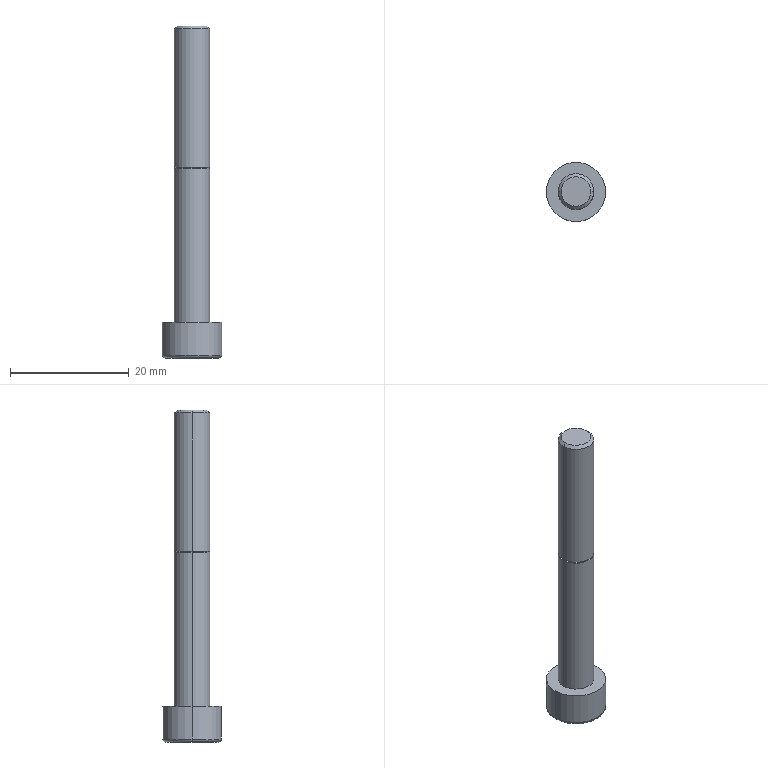Part | SolidWorks | features Attribute 1, Cut 1, Revolution 1 | 1 solid | 27 faces | box 10 x 10 x 56 mm | volume 1826 mm3 | plane 11 | torus 6 | cylinder 6 | cone 4 | commonest cylinder face diameters 6 x4 10 x2
STEP:
#1=CARTESIAN_POINT('',(-2.613,0.,26.01));
#2=VERTEX_POINT('',#1);
#3=CARTESIAN_POINT('',(-2.593,0.,26.03));
#4=VERTEX_POINT('',#3);
#5=CARTESIAN_POINT('',(-2.613,0.,26.03));
#6=DIRECTION('',(0.,-1.,0.));
#7=DIRECTION('',(0.,0.,-1.));
#8=AXIS2_PLACEMENT_3D('',#5,#6,#7);
#9=CIRCLE('',#8,0.02);
#10=EDGE_CURVE('',#2,#4,#9,.T.);
#11=ORIENTED_EDGE('',*,*,#10,.T.);
#12=CARTESIAN_POINT('',(2.593,0.,26.03));
#13=VERTEX_POINT('',#12);
#14=CARTESIAN_POINT('',(0.,0.,26.03));
#15=DIRECTION('',(0.,0.,-1.));
#16=DIRECTION('',(-1.,0.,0.));
#17=AXIS2_PLACEMENT_3D('',#14,#15,#16);
#18=CIRCLE('',#17,2.593);
#19=EDGE_CURVE('',#4,#13,#18,.T.);
#20=ORIENTED_EDGE('',*,*,#19,.T.);
#21=CARTESIAN_POINT('',(2.613,0.,26.01));
#22=VERTEX_POINT('',#21);
#23=CARTESIAN_POINT('',(2.613,0.,26.03));
#24=DIRECTION('',(0.,1.,0.));
#25=DIRECTION('',(-1.,0.,0.));
#26=AXIS2_PLACEMENT_3D('',#23,#24,#25);
#27=CIRCLE('',#26,0.02);
#28=EDGE_CURVE('',#22,#13,#27,.T.);
#29=ORIENTED_EDGE('',*,*,#28,.F.);
#30=CARTESIAN_POINT('',(0.,0.,26.01));
#31=DIRECTION('',(0.,0.,-1.));
#32=DIRECTION('',(-1.,0.,0.));
#33=AXIS2_PLACEMENT_3D('',#30,#31,#32);
#34=CIRCLE('',#33,2.613);
#35=EDGE_CURVE('',#2,#22,#34,.T.);
#36=ORIENTED_EDGE('',*,*,#35,.F.);
#37=EDGE_LOOP('',(#11,#20,#29,#36));
#38=FACE_OUTER_BOUND('',#37,.T.);
#39=CARTESIAN_POINT('',(0.,0.,26.03));
#40=DIRECTION('',(0.,0.,-1.));
#41=DIRECTION('',(-1.,0.,0.));
#42=AXIS2_PLACEMENT_3D('',#39,#40,#41);
#43=TOROIDAL_SURFACE('',#42,2.613,0.02);
#44=ADVANCED_FACE('',(#38),#43,.F.);
#45=ORIENTED_EDGE('',*,*,#28,.T.);
#46=CARTESIAN_POINT('',(0.,0.,26.03));
#47=DIRECTION('',(0.,0.,-1.));
#48=DIRECTION('',(-1.,0.,0.));
#49=AXIS2_PLACEMENT_3D('',#46,#47,#48);
#50=CIRCLE('',#49,2.593);
#51=EDGE_CURVE('',#13,#4,#50,.T.);
#52=ORIENTED_EDGE('',*,*,#51,.T.);
#53=ORIENTED_EDGE('',*,*,#10,.F.);
#54=CARTESIAN_POINT('',(0.,0.,26.01));
#55=DIRECTION('',(0.,0.,-1.));
#56=DIRECTION('',(-1.,0.,0.));
#57=AXIS2_PLACEMENT_3D('',#54,#55,#56);
#58=CIRCLE('',#57,2.613);
#59=EDGE_CURVE('',#22,#2,#58,.T.);
#60=ORIENTED_EDGE('',*,*,#59,.F.);
#61=EDGE_LOOP('',(#45,#52,#53,#60));
#62=FACE_OUTER_BOUND('',#61,.T.);
#63=CARTESIAN_POINT('',(0.,0.,26.03));
#64=DIRECTION('',(0.,0.,-1.));
#65=DIRECTION('',(-1.,0.,0.));
#66=AXIS2_PLACEMENT_3D('',#63,#64,#65);
#67=TOROIDAL_SURFACE('',#66,2.613,0.02);
#68=ADVANCED_FACE('',(#62),#67,.F.);
#69=CARTESIAN_POINT('',(-2.5,0.,50.));
#70=VERTEX_POINT('',#69);
#71=CARTESIAN_POINT('',(2.5,0.,50.));
#72=VERTEX_POINT('',#71);
#73=CARTESIAN_POINT('',(0.,0.,50.));
#74=DIRECTION('',(0.,0.,-1.));
#75=DIRECTION('',(-1.,0.,0.));
#76=AXIS2_PLACEMENT_3D('',#73,#74,#75);
#77=CIRCLE('',#76,2.5);
#78=EDGE_CURVE('',#70,#72,#77,.T.);
#79=ORIENTED_EDGE('',*,*,#78,.T.);
#80=CARTESIAN_POINT('',(3.,0.,49.5));
#81=VERTEX_POINT('',#80);
#82=CARTESIAN_POINT('',(2.5,0.,50.));
#83=DIRECTION('',(0.7071,0.,-0.7071));
#84=VECTOR('',#83,1000.);
#85=LINE('',#82,#84);
#86=EDGE_CURVE('',#72,#81,#85,.T.);
#87=ORIENTED_EDGE('',*,*,#86,.T.);
#88=CARTESIAN_POINT('',(-3.,0.,49.5));
#89=VERTEX_POINT('',#88);
#90=CARTESIAN_POINT('',(0.,0.,49.5));
#91=DIRECTION('',(0.,0.,-1.));
#92=DIRECTION('',(-1.,0.,0.));
#93=AXIS2_PLACEMENT_3D('',#90,#91,#92);
#94=CIRCLE('',#93,3.);
#95=EDGE_CURVE('',#89,#81,#94,.T.);
#96=ORIENTED_EDGE('',*,*,#95,.F.);
#97=CARTESIAN_POINT('',(-2.5,0.,50.));
#98=DIRECTION('',(-0.7071,0.,-0.7071));
#99=VECTOR('',#98,1000.);
#100=LINE('',#97,#99);
#101=EDGE_CURVE('',#70,#89,#100,.T.);
#102=ORIENTED_EDGE('',*,*,#101,.F.);
#103=EDGE_LOOP('',(#79,#87,#96,#102));
#104=FACE_OUTER_BOUND('',#103,.T.);
#105=CARTESIAN_POINT('',(0.,0.,50.));
#106=DIRECTION('',(0.,0.,-1.));
#107=DIRECTION('',(-1.,0.,0.));
#108=AXIS2_PLACEMENT_3D('',#105,#106,#107);
#109=CONICAL_SURFACE('',#108,2.5,0.7854);
#110=ADVANCED_FACE('',(#104),#109,.T.);
#111=ORIENTED_EDGE('',*,*,#95,.T.);
#112=CARTESIAN_POINT('',(3.,0.,26.192));
#113=VERTEX_POINT('',#112);
#114=CARTESIAN_POINT('',(3.,0.,-10.585));
#115=DIRECTION('',(0.,0.,-1.));
#116=VECTOR('',#115,1000.);
#117=LINE('',#114,#116);
#118=EDGE_CURVE('',#81,#113,#117,.T.);
#119=ORIENTED_EDGE('',*,*,#118,.T.);
#120=CARTESIAN_POINT('',(-3.,0.,26.192));
#121=VERTEX_POINT('',#120);
#122=CARTESIAN_POINT('',(0.,0.,26.192));
#123=DIRECTION('',(0.,0.,-1.));
#124=DIRECTION('',(-1.,0.,0.));
#125=AXIS2_PLACEMENT_3D('',#122,#123,#124);
#126=CIRCLE('',#125,3.);
#127=EDGE_CURVE('',#121,#113,#126,.T.);
#128=ORIENTED_EDGE('',*,*,#127,.F.);
#129=CARTESIAN_POINT('',(-3.,0.,-10.585));
#130=DIRECTION('',(0.,0.,-1.));
#131=VECTOR('',#130,1000.);
#132=LINE('',#129,#131);
#133=EDGE_CURVE('',#89,#121,#132,.T.);
#134=ORIENTED_EDGE('',*,*,#133,.F.);
#135=EDGE_LOOP('',(#111,#119,#128,#134));
#136=FACE_OUTER_BOUND('',#135,.T.);
#137=CARTESIAN_POINT('',(0.,0.,-10.585));
#138=DIRECTION('',(0.,0.,-1.));
#139=DIRECTION('',(-1.,0.,0.));
#140=AXIS2_PLACEMENT_3D('',#137,#138,#139);
#141=CYLINDRICAL_SURFACE('',#140,3.);
#142=ADVANCED_FACE('',(#136),#141,.T.);
#143=CARTESIAN_POINT('',(-2.607,0.,26.049));
#144=VERTEX_POINT('',#143);
#145=CARTESIAN_POINT('',(2.607,0.,26.049));
#146=VERTEX_POINT('',#145);
#147=CARTESIAN_POINT('',(0.,0.,26.049));
#148=DIRECTION('',(0.,0.,-1.));
#149=DIRECTION('',(-1.,0.,0.));
#150=AXIS2_PLACEMENT_3D('',#147,#148,#149);
#151=CIRCLE('',#150,2.607);
#152=EDGE_CURVE('',#144,#146,#151,.T.);
#153=ORIENTED_EDGE('',*,*,#152,.F.);
#154=CARTESIAN_POINT('',(-3.,0.,26.192));
#155=DIRECTION('',(-0.9397,0.,0.342));
#156=VECTOR('',#155,1000.);
#157=LINE('',#154,#156);
#158=EDGE_CURVE('',#144,#121,#157,.T.);
#159=ORIENTED_EDGE('',*,*,#158,.T.);
#160=ORIENTED_EDGE('',*,*,#127,.T.);
#161=CARTESIAN_POINT('',(3.,0.,26.192));
#162=DIRECTION('',(0.9397,0.,0.342));
#163=VECTOR('',#162,1000.);
#164=LINE('',#161,#163);
#165=EDGE_CURVE('',#146,#113,#164,.T.);
#166=ORIENTED_EDGE('',*,*,#165,.F.);
#167=EDGE_LOOP('',(#153,#159,#160,#166));
#168=FACE_OUTER_BOUND('',#167,.T.);
#169=CARTESIAN_POINT('',(0.,0.,26.192));
#170=DIRECTION('',(0.,0.,1.));
#171=DIRECTION('',(1.,0.,0.));
#172=AXIS2_PLACEMENT_3D('',#169,#170,#171);
#173=CONICAL_SURFACE('',#172,3.,1.222);
#174=ADVANCED_FACE('',(#168),#173,.T.);
#175=ORIENTED_EDGE('',*,*,#51,.F.);
#176=CARTESIAN_POINT('',(2.613,0.,26.03));
#177=DIRECTION('',(0.,1.,0.));
#178=DIRECTION('',(-1.,0.,0.));
#179=AXIS2_PLACEMENT_3D('',#176,#177,#178);
#180=CIRCLE('',#179,0.02);
#181=EDGE_CURVE('',#13,#146,#180,.T.);
#182=ORIENTED_EDGE('',*,*,#181,.T.);
#183=CARTESIAN_POINT('',(0.,0.,26.049));
#184=DIRECTION('',(0.,0.,-1.));
#185=DIRECTION('',(-1.,0.,0.));
#186=AXIS2_PLACEMENT_3D('',#183,#184,#185);
#187=CIRCLE('',#186,2.607);
#188=EDGE_CURVE('',#146,#144,#187,.T.);
#189=ORIENTED_EDGE('',*,*,#188,.T.);
#190=CARTESIAN_POINT('',(-2.613,0.,26.03));
#191=DIRECTION('',(0.,-1.,0.));
#192=DIRECTION('',(0.,0.,-1.));
#193=AXIS2_PLACEMENT_3D('',#190,#191,#192);
#194=CIRCLE('',#193,0.02);
#195=EDGE_CURVE('',#4,#144,#194,.T.);
#196=ORIENTED_EDGE('',*,*,#195,.F.);
#197=EDGE_LOOP('',(#175,#182,#189,#196));
#198=FACE_OUTER_BOUND('',#197,.T.);
#199=CARTESIAN_POINT('',(0.,0.,26.03));
#200=DIRECTION('',(0.,0.,-1.));
#201=DIRECTION('',(-1.,0.,0.));
#202=AXIS2_PLACEMENT_3D('',#199,#200,#201);
#203=TOROIDAL_SURFACE('',#202,2.613,0.02);
#204=ADVANCED_FACE('',(#198),#203,.F.);
#205=CARTESIAN_POINT('',(-3.,0.,26.01));
#206=VERTEX_POINT('',#205);
#207=CARTESIAN_POINT('',(3.,0.,26.01));
#208=VERTEX_POINT('',#207);
#209=CARTESIAN_POINT('',(0.,0.,26.01));
#210=DIRECTION('',(0.,0.,-1.));
#211=DIRECTION('',(-1.,0.,0.));
#212=AXIS2_PLACEMENT_3D('',#209,#210,#211);
#213=CIRCLE('',#212,3.);
#214=EDGE_CURVE('',#206,#208,#213,.T.);
#215=ORIENTED_EDGE('',*,*,#214,.T.);
#216=CARTESIAN_POINT('',(3.,0.,0.));
#217=VERTEX_POINT('',#216);
#218=CARTESIAN_POINT('',(3.,0.,-10.585));
#219=DIRECTION('',(0.,0.,-1.));
#220=VECTOR('',#219,1000.);
#221=LINE('',#218,#220);
#222=EDGE_CURVE('',#208,#217,#221,.T.);
#223=ORIENTED_EDGE('',*,*,#222,.T.);
#224=CARTESIAN_POINT('',(-3.,0.,0.));
#225=VERTEX_POINT('',#224);
#226=CARTESIAN_POINT('',(0.,0.,0.));
#227=DIRECTION('',(0.,0.,-1.));
#228=DIRECTION('',(-1.,0.,0.));
#229=AXIS2_PLACEMENT_3D('',#226,#227,#228);
#230=CIRCLE('',#229,3.);
#231=EDGE_CURVE('',#225,#217,#230,.T.);
#232=ORIENTED_EDGE('',*,*,#231,.F.);
#233=CARTESIAN_POINT('',(-3.,0.,-10.585));
#234=DIRECTION('',(0.,0.,-1.));
#235=VECTOR('',#234,1000.);
#236=LINE('',#233,#235);
#237=EDGE_CURVE('',#206,#225,#236,.T.);
#238=ORIENTED_EDGE('',*,*,#237,.F.);
#239=EDGE_LOOP('',(#215,#223,#232,#238));
#240=FACE_OUTER_BOUND('',#239,.T.);
#241=CARTESIAN_POINT('',(0.,0.,-10.585));
#242=DIRECTION('',(0.,0.,-1.));
#243=DIRECTION('',(-1.,0.,0.));
#244=AXIS2_PLACEMENT_3D('',#241,#242,#243);
#245=CYLINDRICAL_SURFACE('',#244,3.);
#246=ADVANCED_FACE('',(#240),#245,.T.);
#247=CARTESIAN_POINT('',(-5.,0.,0.));
#248=VERTEX_POINT('',#247);
#249=CARTESIAN_POINT('',(5.,0.,0.));
#250=VERTEX_POINT('',#249);
#251=CARTESIAN_POINT('',(0.,0.,0.));
#252=DIRECTION('',(0.,0.,-1.));
#253=DIRECTION('',(-1.,0.,0.));
#254=AXIS2_PLACEMENT_3D('',#251,#252,#253);
#255=CIRCLE('',#254,5.);
#256=EDGE_CURVE('',#248,#250,#255,.T.);
#257=ORIENTED_EDGE('',*,*,#256,.T.);
#258=CARTESIAN_POINT('',(5.,0.,-5.5));
#259=VERTEX_POINT('',#258);
#260=CARTESIAN_POINT('',(5.,0.,-10.585));
#261=DIRECTION('',(0.,0.,-1.));
#262=VECTOR('',#261,1000.);
#263=LINE('',#260,#262);
#264=EDGE_CURVE('',#250,#259,#263,.T.);
#265=ORIENTED_EDGE('',*,*,#264,.T.);
#266=CARTESIAN_POINT('',(-5.,0.,-5.5));
#267=VERTEX_POINT('',#266);
#268=CARTESIAN_POINT('',(0.,0.,-5.5));
#269=DIRECTION('',(0.,0.,-1.));
#270=DIRECTION('',(-1.,0.,0.));
#271=AXIS2_PLACEMENT_3D('',#268,#269,#270);
#272=CIRCLE('',#271,5.);
#273=EDGE_CURVE('',#267,#259,#272,.T.);
#274=ORIENTED_EDGE('',*,*,#273,.F.);
#275=CARTESIAN_POINT('',(-5.,0.,-10.585));
#276=DIRECTION('',(0.,0.,-1.));
#277=VECTOR('',#276,1000.);
#278=LINE('',#275,#277);
#279=EDGE_CURVE('',#248,#267,#278,.T.);
#280=ORIENTED_EDGE('',*,*,#279,.F.);
#281=EDGE_LOOP('',(#257,#265,#274,#280));
#282=FACE_OUTER_BOUND('',#281,.T.);
#283=CARTESIAN_POINT('',(0.,0.,-10.585));
#284=DIRECTION('',(0.,0.,-1.));
#285=DIRECTION('',(-1.,0.,0.));
#286=AXIS2_PLACEMENT_3D('',#283,#284,#285);
#287=CYLINDRICAL_SURFACE('',#286,5.);
#288=ADVANCED_FACE('',(#282),#287,.T.);
#289=ORIENTED_EDGE('',*,*,#273,.T.);
#290=CARTESIAN_POINT('',(4.5,0.,-6.));
#291=VERTEX_POINT('',#290);
#292=CARTESIAN_POINT('',(4.5,0.,-5.5));
#293=DIRECTION('',(0.,1.,0.));
#294=DIRECTION('',(-1.,0.,0.));
#295=AXIS2_PLACEMENT_3D('',#292,#293,#294);
#296=CIRCLE('',#295,0.5);
#297=EDGE_CURVE('',#259,#291,#296,.T.);
#298=ORIENTED_EDGE('',*,*,#297,.T.);
#299=CARTESIAN_POINT('',(-4.5,0.,-6.));
#300=VERTEX_POINT('',#299);
#301=CARTESIAN_POINT('',(0.,0.,-6.));
#302=DIRECTION('',(0.,0.,-1.));
#303=DIRECTION('',(-1.,0.,0.));
#304=AXIS2_PLACEMENT_3D('',#301,#302,#303);
#305=CIRCLE('',#304,4.5);
#306=EDGE_CURVE('',#300,#291,#305,.T.);
#307=ORIENTED_EDGE('',*,*,#306,.F.);
#308=CARTESIAN_POINT('',(-4.5,0.,-5.5));
#309=DIRECTION('',(0.,-1.,0.));
#310=DIRECTION('',(0.,0.,-1.));
#311=AXIS2_PLACEMENT_3D('',#308,#309,#310);
#312=CIRCLE('',#311,0.5);
#313=EDGE_CURVE('',#267,#300,#312,.T.);
#314=ORIENTED_EDGE('',*,*,#313,.F.);
#315=EDGE_LOOP('',(#289,#298,#307,#314));
#316=FACE_OUTER_BOUND('',#315,.T.);
#317=CARTESIAN_POINT('',(0.,0.,-5.5));
#318=DIRECTION('',(0.,0.,-1.));
#319=DIRECTION('',(-1.,0.,0.));
#320=AXIS2_PLACEMENT_3D('',#317,#318,#319);
#321=TOROIDAL_SURFACE('',#320,4.5,0.5);
#322=ADVANCED_FACE('',(#316),#321,.T.);
#323=ORIENTED_EDGE('',*,*,#297,.F.);
#324=CARTESIAN_POINT('',(0.,0.,-5.5));
#325=DIRECTION('',(0.,0.,-1.));
#326=DIRECTION('',(-1.,0.,0.));
#327=AXIS2_PLACEMENT_3D('',#324,#325,#326);
#328=CIRCLE('',#327,5.);
#329=EDGE_CURVE('',#259,#267,#328,.T.);
#330=ORIENTED_EDGE('',*,*,#329,.T.);
#331=ORIENTED_EDGE('',*,*,#313,.T.);
#332=CARTESIAN_POINT('',(0.,0.,-6.));
#333=DIRECTION('',(0.,0.,-1.));
#334=DIRECTION('',(-1.,0.,0.));
#335=AXIS2_PLACEMENT_3D('',#332,#333,#334);
#336=CIRCLE('',#335,4.5);
#337=EDGE_CURVE('',#291,#300,#336,.T.);
#338=ORIENTED_EDGE('',*,*,#337,.F.);
#339=EDGE_LOOP('',(#323,#330,#331,#338));
#340=FACE_OUTER_BOUND('',#339,.T.);
#341=CARTESIAN_POINT('',(0.,0.,-5.5));
#342=DIRECTION('',(0.,0.,-1.));
#343=DIRECTION('',(-1.,0.,0.));
#344=AXIS2_PLACEMENT_3D('',#341,#342,#343);
#345=TOROIDAL_SURFACE('',#344,4.5,0.5);
#346=ADVANCED_FACE('',(#340),#345,.T.);
#347=ORIENTED_EDGE('',*,*,#264,.F.);
#348=CARTESIAN_POINT('',(0.,0.,0.));
#349=DIRECTION('',(0.,0.,-1.));
#350=DIRECTION('',(-1.,0.,0.));
#351=AXIS2_PLACEMENT_3D('',#348,#349,#350);
#352=CIRCLE('',#351,5.);
#353=EDGE_CURVE('',#250,#248,#352,.T.);
#354=ORIENTED_EDGE('',*,*,#353,.T.);
#355=ORIENTED_EDGE('',*,*,#279,.T.);
#356=ORIENTED_EDGE('',*,*,#329,.F.);
#357=EDGE_LOOP('',(#347,#354,#355,#356));
#358=FACE_OUTER_BOUND('',#357,.T.);
#359=CARTESIAN_POINT('',(0.,0.,-10.585));
#360=DIRECTION('',(0.,0.,-1.));
#361=DIRECTION('',(-1.,0.,0.));
#362=AXIS2_PLACEMENT_3D('',#359,#360,#361);
#363=CYLINDRICAL_SURFACE('',#362,5.);
#364=ADVANCED_FACE('',(#358),#363,.T.);
#365=ORIENTED_EDGE('',*,*,#256,.F.);
#366=ORIENTED_EDGE('',*,*,#353,.F.);
#367=EDGE_LOOP('',(#365,#366));
#368=FACE_OUTER_BOUND('',#367,.T.);
#369=ORIENTED_EDGE('',*,*,#231,.T.);
#370=CARTESIAN_POINT('',(0.,0.,0.));
#371=DIRECTION('',(0.,0.,-1.));
#372=DIRECTION('',(-1.,0.,0.));
#373=AXIS2_PLACEMENT_3D('',#370,#371,#372);
#374=CIRCLE('',#373,3.);
#375=EDGE_CURVE('',#217,#225,#374,.T.);
#376=ORIENTED_EDGE('',*,*,#375,.T.);
#377=EDGE_LOOP('',(#369,#376));
#378=FACE_BOUND('',#377,.T.);
#379=CARTESIAN_POINT('',(-5.,0.,0.));
#380=DIRECTION('',(0.,0.,-1.));
#381=DIRECTION('',(-1.,0.,0.));
#382=AXIS2_PLACEMENT_3D('',#379,#380,#381);
#383=PLANE('',#382);
#384=ADVANCED_FACE('',(#368,#378),#383,.F.);
#385=ORIENTED_EDGE('',*,*,#222,.F.);
#386=CARTESIAN_POINT('',(0.,0.,26.01));
#387=DIRECTION('',(0.,0.,-1.));
#388=DIRECTION('',(-1.,0.,0.));
#389=AXIS2_PLACEMENT_3D('',#386,#387,#388);
#390=CIRCLE('',#389,3.);
#391=EDGE_CURVE('',#208,#206,#390,.T.);
#392=ORIENTED_EDGE('',*,*,#391,.T.);
#393=ORIENTED_EDGE('',*,*,#237,.T.);
#394=ORIENTED_EDGE('',*,*,#375,.F.);
#395=EDGE_LOOP('',(#385,#392,#393,#394));
#396=FACE_OUTER_BOUND('',#395,.T.);
#397=CARTESIAN_POINT('',(0.,0.,-10.585));
#398=DIRECTION('',(0.,0.,-1.));
#399=DIRECTION('',(-1.,0.,0.));
#400=AXIS2_PLACEMENT_3D('',#397,#398,#399);
#401=CYLINDRICAL_SURFACE('',#400,3.);
#402=ADVANCED_FACE('',(#396),#401,.T.);
#403=ORIENTED_EDGE('',*,*,#214,.F.);
#404=ORIENTED_EDGE('',*,*,#391,.F.);
#405=EDGE_LOOP('',(#403,#404));
#406=FACE_OUTER_BOUND('',#405,.T.);
#407=ORIENTED_EDGE('',*,*,#35,.T.);
#408=ORIENTED_EDGE('',*,*,#59,.T.);
#409=EDGE_LOOP('',(#407,#408));
#410=FACE_BOUND('',#409,.T.);
#411=CARTESIAN_POINT('',(-3.,0.,26.01));
#412=DIRECTION('',(0.,0.,-1.));
#413=DIRECTION('',(-1.,0.,0.));
#414=AXIS2_PLACEMENT_3D('',#411,#412,#413);
#415=PLANE('',#414);
#416=ADVANCED_FACE('',(#406,#410),#415,.F.);
#417=ORIENTED_EDGE('',*,*,#19,.F.);
#418=ORIENTED_EDGE('',*,*,#195,.T.);
#419=ORIENTED_EDGE('',*,*,#152,.T.);
#420=ORIENTED_EDGE('',*,*,#181,.F.);
#421=EDGE_LOOP('',(#417,#418,#419,#420));
#422=FACE_OUTER_BOUND('',#421,.T.);
#423=CARTESIAN_POINT('',(0.,0.,26.03));
#424=DIRECTION('',(0.,0.,-1.));
#425=DIRECTION('',(-1.,0.,0.));
#426=AXIS2_PLACEMENT_3D('',#423,#424,#425);
#427=TOROIDAL_SURFACE('',#426,2.613,0.02);
#428=ADVANCED_FACE('',(#422),#427,.F.);
#429=ORIENTED_EDGE('',*,*,#158,.F.);
#430=ORIENTED_EDGE('',*,*,#188,.F.);
#431=ORIENTED_EDGE('',*,*,#165,.T.);
#432=CARTESIAN_POINT('',(0.,0.,26.192));
#433=DIRECTION('',(0.,0.,-1.));
#434=DIRECTION('',(-1.,0.,0.));
#435=AXIS2_PLACEMENT_3D('',#432,#433,#434);
#436=CIRCLE('',#435,3.);
#437=EDGE_CURVE('',#113,#121,#436,.T.);
#438=ORIENTED_EDGE('',*,*,#437,.T.);
#439=EDGE_LOOP('',(#429,#430,#431,#438));
#440=FACE_OUTER_BOUND('',#439,.T.);
#441=CARTESIAN_POINT('',(0.,0.,26.192));
#442=DIRECTION('',(0.,0.,1.));
#443=DIRECTION('',(1.,0.,0.));
#444=AXIS2_PLACEMENT_3D('',#441,#442,#443);
#445=CONICAL_SURFACE('',#444,3.,1.222);
#446=ADVANCED_FACE('',(#440),#445,.T.);
#447=ORIENTED_EDGE('',*,*,#118,.F.);
#448=CARTESIAN_POINT('',(0.,0.,49.5));
#449=DIRECTION('',(0.,0.,-1.));
#450=DIRECTION('',(-1.,0.,0.));
#451=AXIS2_PLACEMENT_3D('',#448,#449,#450);
#452=CIRCLE('',#451,3.);
#453=EDGE_CURVE('',#81,#89,#452,.T.);
#454=ORIENTED_EDGE('',*,*,#453,.T.);
#455=ORIENTED_EDGE('',*,*,#133,.T.);
#456=ORIENTED_EDGE('',*,*,#437,.F.);
#457=EDGE_LOOP('',(#447,#454,#455,#456));
#458=FACE_OUTER_BOUND('',#457,.T.);
#459=CARTESIAN_POINT('',(0.,0.,-10.585));
#460=DIRECTION('',(0.,0.,-1.));
#461=DIRECTION('',(-1.,0.,0.));
#462=AXIS2_PLACEMENT_3D('',#459,#460,#461);
#463=CYLINDRICAL_SURFACE('',#462,3.);
#464=ADVANCED_FACE('',(#458),#463,.T.);
#465=ORIENTED_EDGE('',*,*,#86,.F.);
#466=CARTESIAN_POINT('',(0.,0.,50.));
#467=DIRECTION('',(0.,0.,-1.));
#468=DIRECTION('',(-1.,0.,0.));
#469=AXIS2_PLACEMENT_3D('',#466,#467,#468);
#470=CIRCLE('',#469,2.5);
#471=EDGE_CURVE('',#72,#70,#470,.T.);
#472=ORIENTED_EDGE('',*,*,#471,.T.);
#473=ORIENTED_EDGE('',*,*,#101,.T.);
#474=ORIENTED_EDGE('',*,*,#453,.F.);
#475=EDGE_LOOP('',(#465,#472,#473,#474));
#476=FACE_OUTER_BOUND('',#475,.T.);
#477=CARTESIAN_POINT('',(0.,0.,50.));
#478=DIRECTION('',(0.,0.,-1.));
#479=DIRECTION('',(-1.,0.,0.));
#480=AXIS2_PLACEMENT_3D('',#477,#478,#479);
#481=CONICAL_SURFACE('',#480,2.5,0.7854);
#482=ADVANCED_FACE('',(#476),#481,.T.);
#483=ORIENTED_EDGE('',*,*,#78,.F.);
#484=ORIENTED_EDGE('',*,*,#471,.F.);
#485=EDGE_LOOP('',(#483,#484));
#486=FACE_OUTER_BOUND('',#485,.T.);
#487=CARTESIAN_POINT('',(-2.5,0.,50.));
#488=DIRECTION('',(0.,0.,-1.));
#489=DIRECTION('',(-1.,0.,0.));
#490=AXIS2_PLACEMENT_3D('',#487,#488,#489);
#491=PLANE('',#490);
#492=ADVANCED_FACE('',(#486),#491,.F.);
#493=CARTESIAN_POINT('',(2.887,0.,-6.));
#494=VERTEX_POINT('',#493);
#495=CARTESIAN_POINT('',(1.443,-2.5,-6.));
#496=VERTEX_POINT('',#495);
#497=CARTESIAN_POINT('',(2.887,0.,-6.));
#498=DIRECTION('',(-0.5,-0.866,0.));
#499=VECTOR('',#498,1000.);
#500=LINE('',#497,#499);
#501=EDGE_CURVE('',#494,#496,#500,.T.);
#502=ORIENTED_EDGE('',*,*,#501,.F.);
#503=CARTESIAN_POINT('',(1.443,2.5,-6.));
#504=VERTEX_POINT('',#503);
#505=CARTESIAN_POINT('',(1.443,2.5,-6.));
#506=DIRECTION('',(0.5,-0.866,0.));
#507=VECTOR('',#506,1000.);
#508=LINE('',#505,#507);
#509=EDGE_CURVE('',#504,#494,#508,.T.);
#510=ORIENTED_EDGE('',*,*,#509,.F.);
#511=CARTESIAN_POINT('',(-1.443,2.5,-6.));
#512=VERTEX_POINT('',#511);
#513=CARTESIAN_POINT('',(-1.443,2.5,-6.));
#514=DIRECTION('',(1.,0.,0.));
#515=VECTOR('',#514,1000.);
#516=LINE('',#513,#515);
#517=EDGE_CURVE('',#512,#504,#516,.T.);
#518=ORIENTED_EDGE('',*,*,#517,.F.);
#519=CARTESIAN_POINT('',(-2.887,0.,-6.));
#520=VERTEX_POINT('',#519);
#521=CARTESIAN_POINT('',(-2.887,0.,-6.));
#522=DIRECTION('',(0.5,0.866,0.));
#523=VECTOR('',#522,1000.);
#524=LINE('',#521,#523);
#525=EDGE_CURVE('',#520,#512,#524,.T.);
#526=ORIENTED_EDGE('',*,*,#525,.F.);
#527=CARTESIAN_POINT('',(-1.443,-2.5,-6.));
#528=VERTEX_POINT('',#527);
#529=CARTESIAN_POINT('',(-1.443,-2.5,-6.));
#530=DIRECTION('',(-0.5,0.866,0.));
#531=VECTOR('',#530,1000.);
#532=LINE('',#529,#531);
#533=EDGE_CURVE('',#528,#520,#532,.T.);
#534=ORIENTED_EDGE('',*,*,#533,.F.);
#535=CARTESIAN_POINT('',(1.443,-2.5,-6.));
#536=DIRECTION('',(-1.,0.,0.));
#537=VECTOR('',#536,1000.);
#538=LINE('',#535,#537);
#539=EDGE_CURVE('',#496,#528,#538,.T.);
#540=ORIENTED_EDGE('',*,*,#539,.F.);
#541=EDGE_LOOP('',(#502,#510,#518,#526,#534,#540));
#542=FACE_BOUND('',#541,.T.);
#543=ORIENTED_EDGE('',*,*,#306,.T.);
#544=ORIENTED_EDGE('',*,*,#337,.T.);
#545=EDGE_LOOP('',(#543,#544));
#546=FACE_OUTER_BOUND('',#545,.T.);
#547=CARTESIAN_POINT('',(0.,0.,-6.));
#548=DIRECTION('',(0.,0.,1.));
#549=DIRECTION('',(1.,0.,0.));
#550=AXIS2_PLACEMENT_3D('',#547,#548,#549);
#551=PLANE('',#550);
#552=ADVANCED_FACE('',(#542,#546),#551,.F.);
#553=ORIENTED_EDGE('',*,*,#509,.T.);
#554=CARTESIAN_POINT('',(2.887,0.,-3.5));
#555=VERTEX_POINT('',#554);
#556=CARTESIAN_POINT('',(2.887,0.,-3.5));
#557=DIRECTION('',(0.,0.,-1.));
#558=VECTOR('',#557,1000.);
#559=LINE('',#556,#558);
#560=EDGE_CURVE('',#555,#494,#559,.T.);
#561=ORIENTED_EDGE('',*,*,#560,.F.);
#562=CARTESIAN_POINT('',(1.443,2.5,-3.5));
#563=VERTEX_POINT('',#562);
#564=CARTESIAN_POINT('',(1.443,2.5,-3.5));
#565=DIRECTION('',(0.5,-0.866,0.));
#566=VECTOR('',#565,1000.);
#567=LINE('',#564,#566);
#568=EDGE_CURVE('',#563,#555,#567,.T.);
#569=ORIENTED_EDGE('',*,*,#568,.F.);
#570=CARTESIAN_POINT('',(1.443,2.5,-3.5));
#571=DIRECTION('',(0.,0.,-1.));
#572=VECTOR('',#571,1000.);
#573=LINE('',#570,#572);
#574=EDGE_CURVE('',#563,#504,#573,.T.);
#575=ORIENTED_EDGE('',*,*,#574,.T.);
#576=EDGE_LOOP('',(#553,#561,#569,#575));
#577=FACE_OUTER_BOUND('',#576,.T.);
#578=CARTESIAN_POINT('',(1.443,2.5,-3.5));
#579=DIRECTION('',(0.866,0.5,0.));
#580=DIRECTION('',(-0.5,0.866,0.));
#581=AXIS2_PLACEMENT_3D('',#578,#579,#580);
#582=PLANE('',#581);
#583=ADVANCED_FACE('',(#577),#582,.F.);
#584=ORIENTED_EDGE('',*,*,#517,.T.);
#585=ORIENTED_EDGE('',*,*,#574,.F.);
#586=CARTESIAN_POINT('',(-1.443,2.5,-3.5));
#587=VERTEX_POINT('',#586);
#588=CARTESIAN_POINT('',(-1.443,2.5,-3.5));
#589=DIRECTION('',(1.,0.,0.));
#590=VECTOR('',#589,1000.);
#591=LINE('',#588,#590);
#592=EDGE_CURVE('',#587,#563,#591,.T.);
#593=ORIENTED_EDGE('',*,*,#592,.F.);
#594=CARTESIAN_POINT('',(-1.443,2.5,-3.5));
#595=DIRECTION('',(0.,0.,-1.));
#596=VECTOR('',#595,1000.);
#597=LINE('',#594,#596);
#598=EDGE_CURVE('',#587,#512,#597,.T.);
#599=ORIENTED_EDGE('',*,*,#598,.T.);
#600=EDGE_LOOP('',(#584,#585,#593,#599));
#601=FACE_OUTER_BOUND('',#600,.T.);
#602=CARTESIAN_POINT('',(-1.443,2.5,-3.5));
#603=DIRECTION('',(0.,1.,0.));
#604=DIRECTION('',(-1.,0.,0.));
#605=AXIS2_PLACEMENT_3D('',#602,#603,#604);
#606=PLANE('',#605);
#607=ADVANCED_FACE('',(#601),#606,.F.);
#608=ORIENTED_EDGE('',*,*,#525,.T.);
#609=ORIENTED_EDGE('',*,*,#598,.F.);
#610=CARTESIAN_POINT('',(-2.887,0.,-3.5));
#611=VERTEX_POINT('',#610);
#612=CARTESIAN_POINT('',(-2.887,0.,-3.5));
#613=DIRECTION('',(0.5,0.866,0.));
#614=VECTOR('',#613,1000.);
#615=LINE('',#612,#614);
#616=EDGE_CURVE('',#611,#587,#615,.T.);
#617=ORIENTED_EDGE('',*,*,#616,.F.);
#618=CARTESIAN_POINT('',(-2.887,0.,-3.5));
#619=DIRECTION('',(0.,0.,-1.));
#620=VECTOR('',#619,1000.);
#621=LINE('',#618,#620);
#622=EDGE_CURVE('',#611,#520,#621,.T.);
#623=ORIENTED_EDGE('',*,*,#622,.T.);
#624=EDGE_LOOP('',(#608,#609,#617,#623));
#625=FACE_OUTER_BOUND('',#624,.T.);
#626=CARTESIAN_POINT('',(-2.887,0.,-3.5));
#627=DIRECTION('',(-0.866,0.5,0.));
#628=DIRECTION('',(-0.5,-0.866,0.));
#629=AXIS2_PLACEMENT_3D('',#626,#627,#628);
#630=PLANE('',#629);
#631=ADVANCED_FACE('',(#625),#630,.F.);
#632=ORIENTED_EDGE('',*,*,#533,.T.);
#633=ORIENTED_EDGE('',*,*,#622,.F.);
#634=CARTESIAN_POINT('',(-1.443,-2.5,-3.5));
#635=VERTEX_POINT('',#634);
#636=CARTESIAN_POINT('',(-1.443,-2.5,-3.5));
#637=DIRECTION('',(-0.5,0.866,0.));
#638=VECTOR('',#637,1000.);
#639=LINE('',#636,#638);
#640=EDGE_CURVE('',#635,#611,#639,.T.);
#641=ORIENTED_EDGE('',*,*,#640,.F.);
#642=CARTESIAN_POINT('',(-1.443,-2.5,-3.5));
#643=DIRECTION('',(0.,0.,-1.));
#644=VECTOR('',#643,1000.);
#645=LINE('',#642,#644);
#646=EDGE_CURVE('',#635,#528,#645,.T.);
#647=ORIENTED_EDGE('',*,*,#646,.T.);
#648=EDGE_LOOP('',(#632,#633,#641,#647));
#649=FACE_OUTER_BOUND('',#648,.T.);
#650=CARTESIAN_POINT('',(-1.443,-2.5,-3.5));
#651=DIRECTION('',(-0.866,-0.5,0.));
#652=DIRECTION('',(0.5,-0.866,0.));
#653=AXIS2_PLACEMENT_3D('',#650,#651,#652);
#654=PLANE('',#653);
#655=ADVANCED_FACE('',(#649),#654,.F.);
#656=ORIENTED_EDGE('',*,*,#539,.T.);
#657=ORIENTED_EDGE('',*,*,#646,.F.);
#658=CARTESIAN_POINT('',(1.443,-2.5,-3.5));
#659=VERTEX_POINT('',#658);
#660=CARTESIAN_POINT('',(1.443,-2.5,-3.5));
#661=DIRECTION('',(-1.,0.,0.));
#662=VECTOR('',#661,1000.);
#663=LINE('',#660,#662);
#664=EDGE_CURVE('',#659,#635,#663,.T.);
#665=ORIENTED_EDGE('',*,*,#664,.F.);
#666=CARTESIAN_POINT('',(1.443,-2.5,-3.5));
#667=DIRECTION('',(0.,0.,-1.));
#668=VECTOR('',#667,1000.);
#669=LINE('',#666,#668);
#670=EDGE_CURVE('',#659,#496,#669,.T.);
#671=ORIENTED_EDGE('',*,*,#670,.T.);
#672=EDGE_LOOP('',(#656,#657,#665,#671));
#673=FACE_OUTER_BOUND('',#672,.T.);
#674=CARTESIAN_POINT('',(1.443,-2.5,-3.5));
#675=DIRECTION('',(0.,-1.,0.));
#676=DIRECTION('',(0.,0.,-1.));
#677=AXIS2_PLACEMENT_3D('',#674,#675,#676);
#678=PLANE('',#677);
#679=ADVANCED_FACE('',(#673),#678,.F.);
#680=ORIENTED_EDGE('',*,*,#501,.T.);
#681=ORIENTED_EDGE('',*,*,#670,.F.);
#682=CARTESIAN_POINT('',(2.887,0.,-3.5));
#683=DIRECTION('',(-0.5,-0.866,0.));
#684=VECTOR('',#683,1000.);
#685=LINE('',#682,#684);
#686=EDGE_CURVE('',#555,#659,#685,.T.);
#687=ORIENTED_EDGE('',*,*,#686,.F.);
#688=ORIENTED_EDGE('',*,*,#560,.T.);
#689=EDGE_LOOP('',(#680,#681,#687,#688));
#690=FACE_OUTER_BOUND('',#689,.T.);
#691=CARTESIAN_POINT('',(2.887,0.,-3.5));
#692=DIRECTION('',(0.866,-0.5,0.));
#693=DIRECTION('',(0.5,0.866,0.));
#694=AXIS2_PLACEMENT_3D('',#691,#692,#693);
#695=PLANE('',#694);
#696=ADVANCED_FACE('',(#690),#695,.F.);
#697=ORIENTED_EDGE('',*,*,#568,.T.);
#698=ORIENTED_EDGE('',*,*,#686,.T.);
#699=ORIENTED_EDGE('',*,*,#664,.T.);
#700=ORIENTED_EDGE('',*,*,#640,.T.);
#701=ORIENTED_EDGE('',*,*,#616,.T.);
#702=ORIENTED_EDGE('',*,*,#592,.T.);
#703=EDGE_LOOP('',(#697,#698,#699,#700,#701,#702));
#704=FACE_OUTER_BOUND('',#703,.T.);
#705=CARTESIAN_POINT('',(1.443,2.5,-3.5));
#706=DIRECTION('',(0.,0.,1.));
#707=DIRECTION('',(1.,0.,0.));
#708=AXIS2_PLACEMENT_3D('',#705,#706,#707);
#709=PLANE('',#708);
#710=ADVANCED_FACE('',(#704),#709,.F.);
#711=CLOSED_SHELL('',(#44,#68,#110,#142,#174,#204,#246,#288,#322,#346,#364,#384,#402,#416,#428,#446,#464,#482,#492,#552,#583,#607,#631,#655,#679,#696,#710));
#712=MANIFOLD_SOLID_BREP('',#711);
#713=CARTESIAN_POINT('',(0.,0.,0.));
#714=DIRECTION('',(0.,0.,1.));
#715=DIRECTION('',(1.,0.,0.));
#716=AXIS2_PLACEMENT_3D('',#713,#714,#715);
#717=(LENGTH_UNIT()NAMED_UNIT(*)SI_UNIT(.MILLI.,.METRE.));
#718=UNCERTAINTY_MEASURE_WITH_UNIT(LENGTH_MEASURE(0.00001),#717,'','');
#719=(NAMED_UNIT(*)PLANE_ANGLE_UNIT()SI_UNIT($,.RADIAN.));
#720=(NAMED_UNIT(*)SI_UNIT($,.STERADIAN.)SOLID_ANGLE_UNIT());
#721=(GEOMETRIC_REPRESENTATION_CONTEXT(3)GLOBAL_UNCERTAINTY_ASSIGNED_CONTEXT((#718))GLOBAL_UNIT_ASSIGNED_CONTEXT((#717,#719,#720))REPRESENTATION_CONTEXT('',''));
#722=ADVANCED_BREP_SHAPE_REPRESENTATION('',(#712,#716),#721);